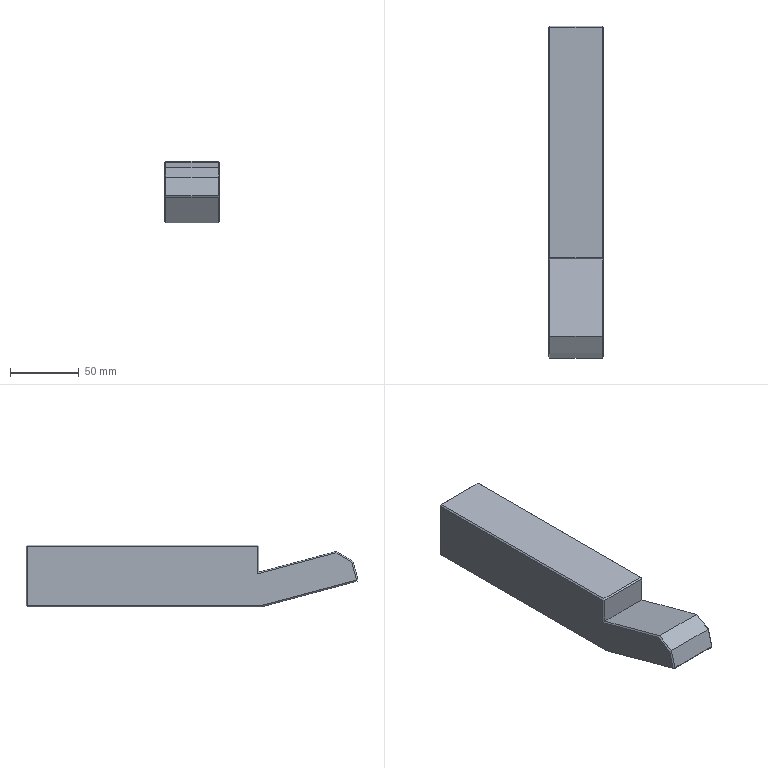Part | STEP file | Cunha 2 - Torre - 2 cav | 1 solid | 46 faces | box 40 x 241.767 x 45 mm | volume 369666 mm3 | plane 38 | cylinder 4 | cone 4 | commonest cylinder face diameters 8.5 x4